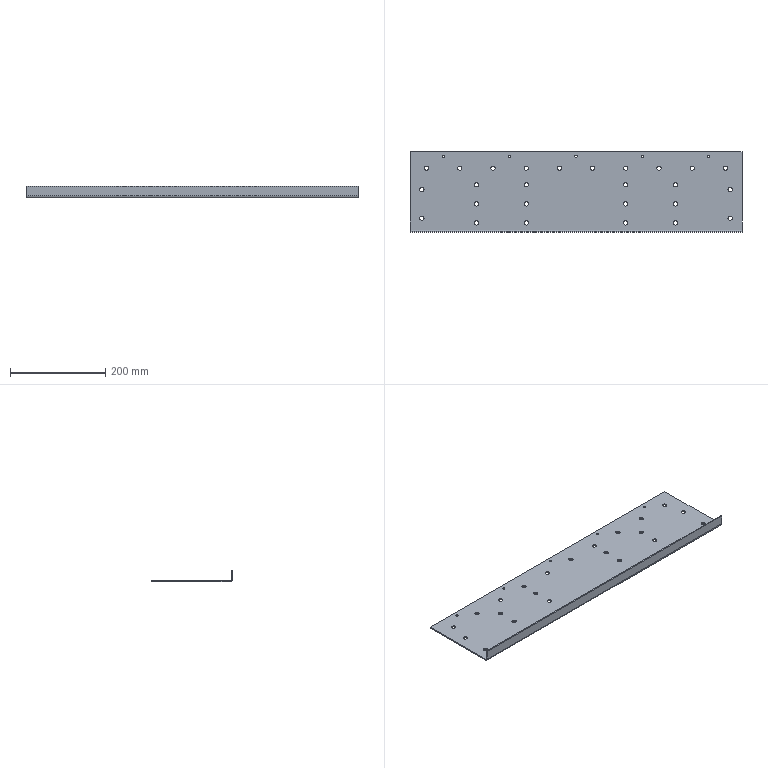Part | STEP file | cc-roller-09 | 1 solid | 41 faces | box 698 x 170 x 25 mm | volume 328733 mm3 | spline 31 | plane 8 | cylinder 2 | commonest cylinder face diameters 5 x1 10 x1